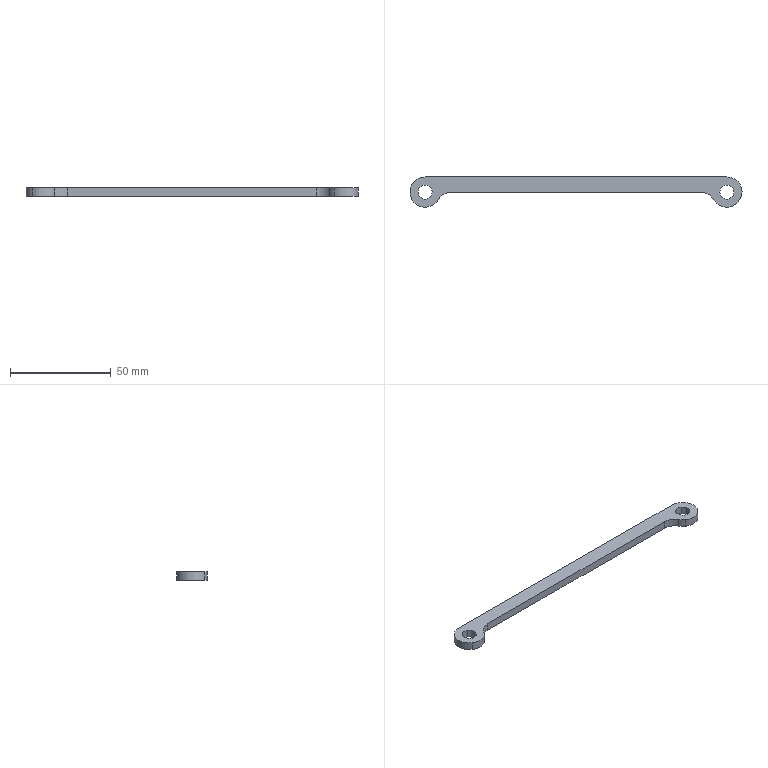Part | NX | features BREP 1 | 1 solid | 15 faces | box 165 x 15 x 4 mm | volume 5289 mm3 | cylinder 11 | plane 4 | commonest cylinder face diameters 15 x7 7 x4
STEP:
#1=CARTESIAN_POINT('',(-9.143,-12.895,7.));
#2=VERTEX_POINT('',#1);
#3=CARTESIAN_POINT('',(-5.209,-7.105,7.));
#4=VERTEX_POINT('',#3);
#5=CARTESIAN_POINT('',(-7.176,-10.,7.));
#6=DIRECTION('',(0.,0.,1.));
#7=DIRECTION('',(1.,0.,0.));
#8=AXIS2_PLACEMENT_3D('',#5,#6,#7);
#9=CIRCLE('',#8,3.5);
#10=EDGE_CURVE('',#2,#4,#9,.T.);
#11=ORIENTED_EDGE('',*,*,#10,.T.);
#12=CARTESIAN_POINT('',(-5.209,-7.105,3.));
#13=VERTEX_POINT('',#12);
#14=CARTESIAN_POINT('',(-5.209,-7.105,6.));
#15=DIRECTION('',(0.,0.,-1.));
#16=VECTOR('',#15,1000.);
#17=LINE('',#14,#16);
#18=EDGE_CURVE('',#13,#4,#17,.F.);
#19=ORIENTED_EDGE('',*,*,#18,.F.);
#20=CARTESIAN_POINT('',(-9.143,-12.895,3.));
#21=VERTEX_POINT('',#20);
#22=CARTESIAN_POINT('',(-7.176,-10.,3.));
#23=DIRECTION('',(0.,0.,1.));
#24=DIRECTION('',(1.,0.,0.));
#25=AXIS2_PLACEMENT_3D('',#22,#23,#24);
#26=CIRCLE('',#25,3.5);
#27=EDGE_CURVE('',#21,#13,#26,.T.);
#28=ORIENTED_EDGE('',*,*,#27,.F.);
#29=CARTESIAN_POINT('',(-9.143,-12.895,6.));
#30=DIRECTION('',(0.,0.,-1.));
#31=VECTOR('',#30,1000.);
#32=LINE('',#29,#31);
#33=EDGE_CURVE('',#21,#2,#32,.F.);
#34=ORIENTED_EDGE('',*,*,#33,.T.);
#35=EDGE_LOOP('',(#11,#19,#28,#34));
#36=FACE_BOUND('',#35,.T.);
#37=CARTESIAN_POINT('',(-7.176,-10.,6.));
#38=DIRECTION('',(0.,0.,-1.));
#39=DIRECTION('',(0.562,0.8271,0.));
#40=AXIS2_PLACEMENT_3D('',#37,#38,#39);
#41=CYLINDRICAL_SURFACE('',#40,3.5);
#42=ADVANCED_FACE('',(#36),#41,.F.);
#43=CARTESIAN_POINT('',(-11.392,-16.203,7.));
#44=VERTEX_POINT('',#43);
#45=CARTESIAN_POINT('',(-0.681,-13.75,7.));
#46=VERTEX_POINT('',#45);
#47=CARTESIAN_POINT('',(-7.176,-10.,7.));
#48=DIRECTION('',(0.,0.,1.));
#49=DIRECTION('',(1.,0.,0.));
#50=AXIS2_PLACEMENT_3D('',#47,#48,#49);
#51=CIRCLE('',#50,7.5);
#52=EDGE_CURVE('',#44,#46,#51,.T.);
#53=ORIENTED_EDGE('',*,*,#52,.F.);
#54=CARTESIAN_POINT('',(-11.392,-16.203,3.));
#55=VERTEX_POINT('',#54);
#56=CARTESIAN_POINT('',(-11.392,-16.203,6.));
#57=DIRECTION('',(0.,0.,-1.));
#58=VECTOR('',#57,1000.);
#59=LINE('',#56,#58);
#60=EDGE_CURVE('',#44,#55,#59,.T.);
#61=ORIENTED_EDGE('',*,*,#60,.T.);
#62=CARTESIAN_POINT('',(-0.681,-13.75,3.));
#63=VERTEX_POINT('',#62);
#64=CARTESIAN_POINT('',(-7.176,-10.,3.));
#65=DIRECTION('',(0.,0.,1.));
#66=DIRECTION('',(1.,0.,0.));
#67=AXIS2_PLACEMENT_3D('',#64,#65,#66);
#68=CIRCLE('',#67,7.5);
#69=EDGE_CURVE('',#55,#63,#68,.T.);
#70=ORIENTED_EDGE('',*,*,#69,.T.);
#71=CARTESIAN_POINT('',(-0.681,-13.75,6.));
#72=DIRECTION('',(0.,0.,1.));
#73=VECTOR('',#72,1000.);
#74=LINE('',#71,#73);
#75=EDGE_CURVE('',#63,#46,#74,.T.);
#76=ORIENTED_EDGE('',*,*,#75,.T.);
#77=EDGE_LOOP('',(#53,#61,#70,#76));
#78=FACE_BOUND('',#77,.T.);
#79=CARTESIAN_POINT('',(-7.176,-10.,6.));
#80=DIRECTION('',(0.,0.,-1.));
#81=DIRECTION('',(0.562,0.8271,0.));
#82=AXIS2_PLACEMENT_3D('',#79,#80,#81);
#83=CYLINDRICAL_SURFACE('',#82,7.5);
#84=ADVANCED_FACE('',(#78),#83,.T.);
#85=CARTESIAN_POINT('',(144.791,-7.105,7.));
#86=VERTEX_POINT('',#85);
#87=CARTESIAN_POINT('',(140.857,-12.895,7.));
#88=VERTEX_POINT('',#87);
#89=CARTESIAN_POINT('',(142.824,-10.,7.));
#90=DIRECTION('',(0.,0.,-1.));
#91=DIRECTION('',(1.,0.,0.));
#92=AXIS2_PLACEMENT_3D('',#89,#90,#91);
#93=CIRCLE('',#92,3.5);
#94=EDGE_CURVE('',#86,#88,#93,.T.);
#95=ORIENTED_EDGE('',*,*,#94,.F.);
#96=CARTESIAN_POINT('',(144.791,-7.105,3.));
#97=VERTEX_POINT('',#96);
#98=CARTESIAN_POINT('',(144.791,-7.105,6.));
#99=DIRECTION('',(0.,0.,-1.));
#100=VECTOR('',#99,1000.);
#101=LINE('',#98,#100);
#102=EDGE_CURVE('',#97,#86,#101,.F.);
#103=ORIENTED_EDGE('',*,*,#102,.F.);
#104=CARTESIAN_POINT('',(140.857,-12.895,3.));
#105=VERTEX_POINT('',#104);
#106=CARTESIAN_POINT('',(142.824,-10.,3.));
#107=DIRECTION('',(0.,0.,1.));
#108=DIRECTION('',(1.,0.,0.));
#109=AXIS2_PLACEMENT_3D('',#106,#107,#108);
#110=CIRCLE('',#109,3.5);
#111=EDGE_CURVE('',#105,#97,#110,.T.);
#112=ORIENTED_EDGE('',*,*,#111,.F.);
#113=CARTESIAN_POINT('',(140.857,-12.895,6.));
#114=DIRECTION('',(0.,0.,-1.));
#115=VECTOR('',#114,1000.);
#116=LINE('',#113,#115);
#117=EDGE_CURVE('',#105,#88,#116,.F.);
#118=ORIENTED_EDGE('',*,*,#117,.T.);
#119=EDGE_LOOP('',(#95,#103,#112,#118));
#120=FACE_BOUND('',#119,.T.);
#121=CARTESIAN_POINT('',(142.824,-10.,6.));
#122=DIRECTION('',(0.,0.,-1.));
#123=DIRECTION('',(0.562,0.8271,0.));
#124=AXIS2_PLACEMENT_3D('',#121,#122,#123);
#125=CYLINDRICAL_SURFACE('',#124,3.5);
#126=ADVANCED_FACE('',(#120),#125,.F.);
#127=CARTESIAN_POINT('',(147.039,-3.797,7.));
#128=VERTEX_POINT('',#127);
#129=CARTESIAN_POINT('',(142.824,-2.5,7.));
#130=VERTEX_POINT('',#129);
#131=CARTESIAN_POINT('',(142.824,-10.,7.));
#132=DIRECTION('',(0.,0.,1.));
#133=DIRECTION('',(1.,0.,0.));
#134=AXIS2_PLACEMENT_3D('',#131,#132,#133);
#135=CIRCLE('',#134,7.5);
#136=EDGE_CURVE('',#128,#130,#135,.T.);
#137=ORIENTED_EDGE('',*,*,#136,.F.);
#138=CARTESIAN_POINT('',(147.039,-3.797,3.));
#139=VERTEX_POINT('',#138);
#140=CARTESIAN_POINT('',(147.039,-3.797,6.));
#141=DIRECTION('',(0.,0.,-1.));
#142=VECTOR('',#141,1000.);
#143=LINE('',#140,#142);
#144=EDGE_CURVE('',#128,#139,#143,.T.);
#145=ORIENTED_EDGE('',*,*,#144,.T.);
#146=CARTESIAN_POINT('',(142.824,-2.5,3.));
#147=VERTEX_POINT('',#146);
#148=CARTESIAN_POINT('',(142.824,-10.,3.));
#149=DIRECTION('',(0.,0.,1.));
#150=DIRECTION('',(1.,0.,0.));
#151=AXIS2_PLACEMENT_3D('',#148,#149,#150);
#152=CIRCLE('',#151,7.5);
#153=EDGE_CURVE('',#139,#147,#152,.T.);
#154=ORIENTED_EDGE('',*,*,#153,.T.);
#155=CARTESIAN_POINT('',(142.824,-2.5,6.));
#156=DIRECTION('',(0.,0.,1.));
#157=VECTOR('',#156,1000.);
#158=LINE('',#155,#157);
#159=EDGE_CURVE('',#147,#130,#158,.T.);
#160=ORIENTED_EDGE('',*,*,#159,.T.);
#161=EDGE_LOOP('',(#137,#145,#154,#160));
#162=FACE_BOUND('',#161,.T.);
#163=CARTESIAN_POINT('',(142.824,-10.,6.));
#164=DIRECTION('',(0.,0.,-1.));
#165=DIRECTION('',(0.562,0.8271,0.));
#166=AXIS2_PLACEMENT_3D('',#163,#164,#165);
#167=CYLINDRICAL_SURFACE('',#166,7.5);
#168=ADVANCED_FACE('',(#162),#167,.T.);
#169=ORIENTED_EDGE('',*,*,#144,.F.);
#170=CARTESIAN_POINT('',(138.608,-16.203,7.));
#171=VERTEX_POINT('',#170);
#172=CARTESIAN_POINT('',(142.824,-10.,7.));
#173=DIRECTION('',(0.,0.,1.));
#174=DIRECTION('',(1.,0.,0.));
#175=AXIS2_PLACEMENT_3D('',#172,#173,#174);
#176=CIRCLE('',#175,7.5);
#177=EDGE_CURVE('',#171,#128,#176,.T.);
#178=ORIENTED_EDGE('',*,*,#177,.F.);
#179=CARTESIAN_POINT('',(138.608,-16.203,3.));
#180=VERTEX_POINT('',#179);
#181=CARTESIAN_POINT('',(138.608,-16.203,6.));
#182=DIRECTION('',(0.,0.,-1.));
#183=VECTOR('',#182,1000.);
#184=LINE('',#181,#183);
#185=EDGE_CURVE('',#171,#180,#184,.T.);
#186=ORIENTED_EDGE('',*,*,#185,.T.);
#187=CARTESIAN_POINT('',(142.824,-10.,3.));
#188=DIRECTION('',(0.,0.,1.));
#189=DIRECTION('',(1.,0.,0.));
#190=AXIS2_PLACEMENT_3D('',#187,#188,#189);
#191=CIRCLE('',#190,7.5);
#192=EDGE_CURVE('',#180,#139,#191,.T.);
#193=ORIENTED_EDGE('',*,*,#192,.T.);
#194=EDGE_LOOP('',(#169,#178,#186,#193));
#195=FACE_BOUND('',#194,.T.);
#196=CARTESIAN_POINT('',(142.824,-10.,6.));
#197=DIRECTION('',(0.,0.,-1.));
#198=DIRECTION('',(0.562,0.8271,0.));
#199=AXIS2_PLACEMENT_3D('',#196,#197,#198);
#200=CYLINDRICAL_SURFACE('',#199,7.5);
#201=ADVANCED_FACE('',(#195),#200,.T.);
#202=ORIENTED_EDGE('',*,*,#185,.F.);
#203=CARTESIAN_POINT('',(136.329,-13.75,7.));
#204=VERTEX_POINT('',#203);
#205=CARTESIAN_POINT('',(142.824,-10.,7.));
#206=DIRECTION('',(0.,0.,1.));
#207=DIRECTION('',(1.,0.,0.));
#208=AXIS2_PLACEMENT_3D('',#205,#206,#207);
#209=CIRCLE('',#208,7.5);
#210=EDGE_CURVE('',#204,#171,#209,.T.);
#211=ORIENTED_EDGE('',*,*,#210,.F.);
#212=CARTESIAN_POINT('',(136.329,-13.75,3.));
#213=VERTEX_POINT('',#212);
#214=CARTESIAN_POINT('',(136.329,-13.75,6.));
#215=DIRECTION('',(0.,0.,-1.));
#216=VECTOR('',#215,1000.);
#217=LINE('',#214,#216);
#218=EDGE_CURVE('',#204,#213,#217,.T.);
#219=ORIENTED_EDGE('',*,*,#218,.T.);
#220=CARTESIAN_POINT('',(142.824,-10.,3.));
#221=DIRECTION('',(0.,0.,1.));
#222=DIRECTION('',(1.,0.,0.));
#223=AXIS2_PLACEMENT_3D('',#220,#221,#222);
#224=CIRCLE('',#223,7.5);
#225=EDGE_CURVE('',#213,#180,#224,.T.);
#226=ORIENTED_EDGE('',*,*,#225,.T.);
#227=EDGE_LOOP('',(#202,#211,#219,#226));
#228=FACE_BOUND('',#227,.T.);
#229=CARTESIAN_POINT('',(142.824,-10.,6.));
#230=DIRECTION('',(0.,0.,-1.));
#231=DIRECTION('',(0.562,0.8271,0.));
#232=AXIS2_PLACEMENT_3D('',#229,#230,#231);
#233=CYLINDRICAL_SURFACE('',#232,7.5);
#234=ADVANCED_FACE('',(#228),#233,.T.);
#235=CARTESIAN_POINT('',(-7.176,-2.5,7.));
#236=VERTEX_POINT('',#235);
#237=CARTESIAN_POINT('',(2.824,-2.5,7.));
#238=DIRECTION('',(-1.,0.,0.));
#239=VECTOR('',#238,1000.);
#240=LINE('',#237,#239);
#241=EDGE_CURVE('',#130,#236,#240,.T.);
#242=ORIENTED_EDGE('',*,*,#241,.T.);
#243=CARTESIAN_POINT('',(-7.176,-10.,7.));
#244=DIRECTION('',(0.,0.,1.));
#245=DIRECTION('',(1.,0.,0.));
#246=AXIS2_PLACEMENT_3D('',#243,#244,#245);
#247=CIRCLE('',#246,7.5);
#248=EDGE_CURVE('',#236,#44,#247,.T.);
#249=ORIENTED_EDGE('',*,*,#248,.T.);
#250=ORIENTED_EDGE('',*,*,#52,.T.);
#251=CARTESIAN_POINT('',(5.814,-10.,7.));
#252=VERTEX_POINT('',#251);
#253=CARTESIAN_POINT('',(5.814,-17.5,7.));
#254=DIRECTION('',(0.,0.,-1.));
#255=DIRECTION('',(1.,0.,0.));
#256=AXIS2_PLACEMENT_3D('',#253,#254,#255);
#257=CIRCLE('',#256,7.5);
#258=EDGE_CURVE('',#46,#252,#257,.T.);
#259=ORIENTED_EDGE('',*,*,#258,.T.);
#260=CARTESIAN_POINT('',(129.833,-10.,7.));
#261=VERTEX_POINT('',#260);
#262=CARTESIAN_POINT('',(2.824,-10.,7.));
#263=DIRECTION('',(-1.,0.,0.));
#264=VECTOR('',#263,1000.);
#265=LINE('',#262,#264);
#266=EDGE_CURVE('',#261,#252,#265,.T.);
#267=ORIENTED_EDGE('',*,*,#266,.F.);
#268=CARTESIAN_POINT('',(129.833,-17.5,7.));
#269=DIRECTION('',(0.,0.,-1.));
#270=DIRECTION('',(1.,0.,0.));
#271=AXIS2_PLACEMENT_3D('',#268,#269,#270);
#272=CIRCLE('',#271,7.5);
#273=EDGE_CURVE('',#261,#204,#272,.T.);
#274=ORIENTED_EDGE('',*,*,#273,.T.);
#275=ORIENTED_EDGE('',*,*,#210,.T.);
#276=ORIENTED_EDGE('',*,*,#177,.T.);
#277=ORIENTED_EDGE('',*,*,#136,.T.);
#278=EDGE_LOOP('',(#242,#249,#250,#259,#267,#274,#275,#276,#277));
#279=FACE_BOUND('',#278,.T.);
#280=CARTESIAN_POINT('',(142.824,-10.,7.));
#281=DIRECTION('',(0.,0.,-1.));
#282=DIRECTION('',(1.,0.,0.));
#283=AXIS2_PLACEMENT_3D('',#280,#281,#282);
#284=CIRCLE('',#283,3.5);
#285=EDGE_CURVE('',#88,#86,#284,.T.);
#286=ORIENTED_EDGE('',*,*,#285,.T.);
#287=ORIENTED_EDGE('',*,*,#94,.T.);
#288=EDGE_LOOP('',(#286,#287));
#289=FACE_BOUND('',#288,.T.);
#290=ORIENTED_EDGE('',*,*,#10,.F.);
#291=CARTESIAN_POINT('',(-7.176,-10.,7.));
#292=DIRECTION('',(0.,0.,1.));
#293=DIRECTION('',(1.,0.,0.));
#294=AXIS2_PLACEMENT_3D('',#291,#292,#293);
#295=CIRCLE('',#294,3.5);
#296=EDGE_CURVE('',#4,#2,#295,.T.);
#297=ORIENTED_EDGE('',*,*,#296,.F.);
#298=EDGE_LOOP('',(#290,#297));
#299=FACE_BOUND('',#298,.T.);
#300=CARTESIAN_POINT('',(2.824,-10.,7.));
#301=DIRECTION('',(0.,0.,1.));
#302=DIRECTION('',(-1.,0.,0.));
#303=AXIS2_PLACEMENT_3D('',#300,#301,#302);
#304=PLANE('',#303);
#305=ADVANCED_FACE('',(#279,#289,#299),#304,.T.);
#306=ORIENTED_EDGE('',*,*,#102,.T.);
#307=ORIENTED_EDGE('',*,*,#285,.F.);
#308=ORIENTED_EDGE('',*,*,#117,.F.);
#309=CARTESIAN_POINT('',(142.824,-10.,3.));
#310=DIRECTION('',(0.,0.,1.));
#311=DIRECTION('',(1.,0.,0.));
#312=AXIS2_PLACEMENT_3D('',#309,#310,#311);
#313=CIRCLE('',#312,3.5);
#314=EDGE_CURVE('',#97,#105,#313,.T.);
#315=ORIENTED_EDGE('',*,*,#314,.F.);
#316=EDGE_LOOP('',(#306,#307,#308,#315));
#317=FACE_BOUND('',#316,.T.);
#318=CARTESIAN_POINT('',(142.824,-10.,6.));
#319=DIRECTION('',(0.,0.,-1.));
#320=DIRECTION('',(0.562,0.8271,0.));
#321=AXIS2_PLACEMENT_3D('',#318,#319,#320);
#322=CYLINDRICAL_SURFACE('',#321,3.5);
#323=ADVANCED_FACE('',(#317),#322,.F.);
#324=CARTESIAN_POINT('',(5.814,-10.,3.));
#325=VERTEX_POINT('',#324);
#326=CARTESIAN_POINT('',(129.833,-10.,3.));
#327=VERTEX_POINT('',#326);
#328=CARTESIAN_POINT('',(135.324,-10.,3.));
#329=DIRECTION('',(1.,0.,0.));
#330=VECTOR('',#329,1000.);
#331=LINE('',#328,#330);
#332=EDGE_CURVE('',#325,#327,#331,.T.);
#333=ORIENTED_EDGE('',*,*,#332,.F.);
#334=CARTESIAN_POINT('',(5.814,-17.5,3.));
#335=DIRECTION('',(0.,0.,1.));
#336=DIRECTION('',(1.,0.,0.));
#337=AXIS2_PLACEMENT_3D('',#334,#335,#336);
#338=CIRCLE('',#337,7.5);
#339=EDGE_CURVE('',#325,#63,#338,.T.);
#340=ORIENTED_EDGE('',*,*,#339,.T.);
#341=ORIENTED_EDGE('',*,*,#69,.F.);
#342=CARTESIAN_POINT('',(-7.176,-2.5,3.));
#343=VERTEX_POINT('',#342);
#344=CARTESIAN_POINT('',(-7.176,-10.,3.));
#345=DIRECTION('',(0.,0.,1.));
#346=DIRECTION('',(1.,0.,0.));
#347=AXIS2_PLACEMENT_3D('',#344,#345,#346);
#348=CIRCLE('',#347,7.5);
#349=EDGE_CURVE('',#343,#55,#348,.T.);
#350=ORIENTED_EDGE('',*,*,#349,.F.);
#351=CARTESIAN_POINT('',(-6.981,-2.5,3.));
#352=DIRECTION('',(1.,0.,0.));
#353=VECTOR('',#352,1000.);
#354=LINE('',#351,#353);
#355=EDGE_CURVE('',#343,#147,#354,.T.);
#356=ORIENTED_EDGE('',*,*,#355,.T.);
#357=ORIENTED_EDGE('',*,*,#153,.F.);
#358=ORIENTED_EDGE('',*,*,#192,.F.);
#359=ORIENTED_EDGE('',*,*,#225,.F.);
#360=CARTESIAN_POINT('',(129.833,-17.5,3.));
#361=DIRECTION('',(0.,0.,1.));
#362=DIRECTION('',(1.,0.,0.));
#363=AXIS2_PLACEMENT_3D('',#360,#361,#362);
#364=CIRCLE('',#363,7.5);
#365=EDGE_CURVE('',#213,#327,#364,.T.);
#366=ORIENTED_EDGE('',*,*,#365,.T.);
#367=EDGE_LOOP('',(#333,#340,#341,#350,#356,#357,#358,#359,#366));
#368=FACE_BOUND('',#367,.T.);
#369=ORIENTED_EDGE('',*,*,#111,.T.);
#370=ORIENTED_EDGE('',*,*,#314,.T.);
#371=EDGE_LOOP('',(#369,#370));
#372=FACE_BOUND('',#371,.T.);
#373=ORIENTED_EDGE('',*,*,#27,.T.);
#374=CARTESIAN_POINT('',(-7.176,-10.,3.));
#375=DIRECTION('',(0.,0.,1.));
#376=DIRECTION('',(1.,0.,0.));
#377=AXIS2_PLACEMENT_3D('',#374,#375,#376);
#378=CIRCLE('',#377,3.5);
#379=EDGE_CURVE('',#13,#21,#378,.T.);
#380=ORIENTED_EDGE('',*,*,#379,.T.);
#381=EDGE_LOOP('',(#373,#380));
#382=FACE_BOUND('',#381,.T.);
#383=CARTESIAN_POINT('',(2.824,-10.,3.));
#384=DIRECTION('',(0.,0.,1.));
#385=DIRECTION('',(-1.,0.,0.));
#386=AXIS2_PLACEMENT_3D('',#383,#384,#385);
#387=PLANE('',#386);
#388=ADVANCED_FACE('',(#368,#372,#382),#387,.F.);
#389=ORIENTED_EDGE('',*,*,#60,.F.);
#390=ORIENTED_EDGE('',*,*,#248,.F.);
#391=CARTESIAN_POINT('',(-7.176,-2.5,6.));
#392=DIRECTION('',(0.,0.,1.));
#393=VECTOR('',#392,1000.);
#394=LINE('',#391,#393);
#395=EDGE_CURVE('',#343,#236,#394,.T.);
#396=ORIENTED_EDGE('',*,*,#395,.F.);
#397=ORIENTED_EDGE('',*,*,#349,.T.);
#398=EDGE_LOOP('',(#389,#390,#396,#397));
#399=FACE_BOUND('',#398,.T.);
#400=CARTESIAN_POINT('',(-7.176,-10.,6.));
#401=DIRECTION('',(0.,0.,-1.));
#402=DIRECTION('',(0.562,0.8271,0.));
#403=AXIS2_PLACEMENT_3D('',#400,#401,#402);
#404=CYLINDRICAL_SURFACE('',#403,7.5);
#405=ADVANCED_FACE('',(#399),#404,.T.);
#406=ORIENTED_EDGE('',*,*,#18,.T.);
#407=ORIENTED_EDGE('',*,*,#296,.T.);
#408=ORIENTED_EDGE('',*,*,#33,.F.);
#409=ORIENTED_EDGE('',*,*,#379,.F.);
#410=EDGE_LOOP('',(#406,#407,#408,#409));
#411=FACE_BOUND('',#410,.T.);
#412=CARTESIAN_POINT('',(-7.176,-10.,6.));
#413=DIRECTION('',(0.,0.,-1.));
#414=DIRECTION('',(0.562,0.8271,0.));
#415=AXIS2_PLACEMENT_3D('',#412,#413,#414);
#416=CYLINDRICAL_SURFACE('',#415,3.5);
#417=ADVANCED_FACE('',(#411),#416,.F.);
#418=ORIENTED_EDGE('',*,*,#266,.T.);
#419=CARTESIAN_POINT('',(5.814,-10.,3.));
#420=DIRECTION('',(0.,0.,-1.));
#421=VECTOR('',#420,1000.);
#422=LINE('',#419,#421);
#423=EDGE_CURVE('',#252,#325,#422,.T.);
#424=ORIENTED_EDGE('',*,*,#423,.T.);
#425=ORIENTED_EDGE('',*,*,#332,.T.);
#426=CARTESIAN_POINT('',(129.833,-10.,7.));
#427=DIRECTION('',(0.,0.,1.));
#428=VECTOR('',#427,1000.);
#429=LINE('',#426,#428);
#430=EDGE_CURVE('',#327,#261,#429,.T.);
#431=ORIENTED_EDGE('',*,*,#430,.T.);
#432=EDGE_LOOP('',(#418,#424,#425,#431));
#433=FACE_BOUND('',#432,.T.);
#434=CARTESIAN_POINT('',(135.324,-10.,13.));
#435=DIRECTION('',(0.,1.,0.));
#436=DIRECTION('',(-1.,0.,0.));
#437=AXIS2_PLACEMENT_3D('',#434,#435,#436);
#438=PLANE('',#437);
#439=ADVANCED_FACE('',(#433),#438,.F.);
#440=ORIENTED_EDGE('',*,*,#159,.F.);
#441=ORIENTED_EDGE('',*,*,#355,.F.);
#442=ORIENTED_EDGE('',*,*,#395,.T.);
#443=ORIENTED_EDGE('',*,*,#241,.F.);
#444=EDGE_LOOP('',(#440,#441,#442,#443));
#445=FACE_BOUND('',#444,.T.);
#446=CARTESIAN_POINT('',(-6.981,-2.5,-153.99));
#447=DIRECTION('',(0.,1.,0.));
#448=DIRECTION('',(-1.,0.,0.));
#449=AXIS2_PLACEMENT_3D('',#446,#447,#448);
#450=PLANE('',#449);
#451=ADVANCED_FACE('',(#445),#450,.T.);
#452=ORIENTED_EDGE('',*,*,#258,.F.);
#453=ORIENTED_EDGE('',*,*,#75,.F.);
#454=ORIENTED_EDGE('',*,*,#339,.F.);
#455=ORIENTED_EDGE('',*,*,#423,.F.);
#456=EDGE_LOOP('',(#452,#453,#454,#455));
#457=FACE_BOUND('',#456,.T.);
#458=CARTESIAN_POINT('',(5.814,-17.5,6.));
#459=DIRECTION('',(0.,0.,-1.));
#460=DIRECTION('',(1.,0.,0.));
#461=AXIS2_PLACEMENT_3D('',#458,#459,#460);
#462=CYLINDRICAL_SURFACE('',#461,7.5);
#463=ADVANCED_FACE('',(#457),#462,.F.);
#464=ORIENTED_EDGE('',*,*,#273,.F.);
#465=ORIENTED_EDGE('',*,*,#430,.F.);
#466=ORIENTED_EDGE('',*,*,#365,.F.);
#467=ORIENTED_EDGE('',*,*,#218,.F.);
#468=EDGE_LOOP('',(#464,#465,#466,#467));
#469=FACE_BOUND('',#468,.T.);
#470=CARTESIAN_POINT('',(129.833,-17.5,6.));
#471=DIRECTION('',(0.,0.,-1.));
#472=DIRECTION('',(1.,0.,0.));
#473=AXIS2_PLACEMENT_3D('',#470,#471,#472);
#474=CYLINDRICAL_SURFACE('',#473,7.5);
#475=ADVANCED_FACE('',(#469),#474,.F.);
#476=CLOSED_SHELL('',(#42,#84,#126,#168,#201,#234,#305,#323,#388,#405,#417,#439,#451,#463,#475));
#477=MANIFOLD_SOLID_BREP('',#476);
#478=(LENGTH_UNIT()NAMED_UNIT(*)SI_UNIT(.MILLI.,.METRE.));
#479=UNCERTAINTY_MEASURE_WITH_UNIT(LENGTH_MEASURE(0.00001),#478,'','');
#480=(NAMED_UNIT(*)PLANE_ANGLE_UNIT()SI_UNIT($,.RADIAN.));
#481=(NAMED_UNIT(*)SI_UNIT($,.STERADIAN.)SOLID_ANGLE_UNIT());
#482=(GEOMETRIC_REPRESENTATION_CONTEXT(3)GLOBAL_UNCERTAINTY_ASSIGNED_CONTEXT((#479))GLOBAL_UNIT_ASSIGNED_CONTEXT((#478,#480,#481))REPRESENTATION_CONTEXT('',''));
#483=ADVANCED_BREP_SHAPE_REPRESENTATION('',(#477),#482);